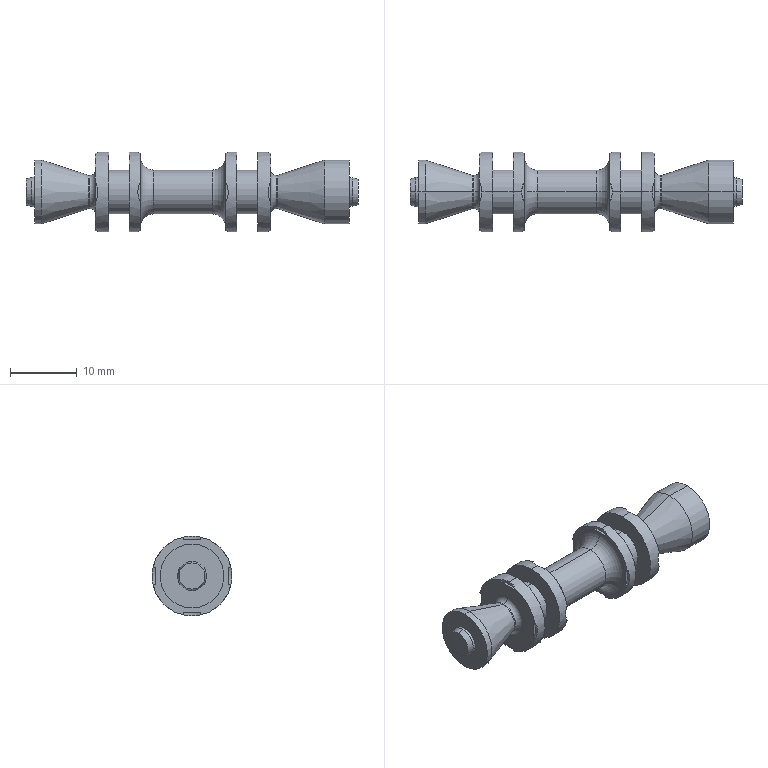Part | SolidWorks | features Fillet 2, Chamfer 1, CirPattern 1, ICE 1, MirrorPattern 1, Revolution 1 | 1 solid | 118 faces | box 49.9 x 12 x 12 mm | volume 2556 mm3 | plane 60 | cylinder 42 | cone 8 | torus 8 | commonest cylinder face diameters 7.01 x16 12 x8 6.6 x6 5 x4 9.6 x4 4.3 x2